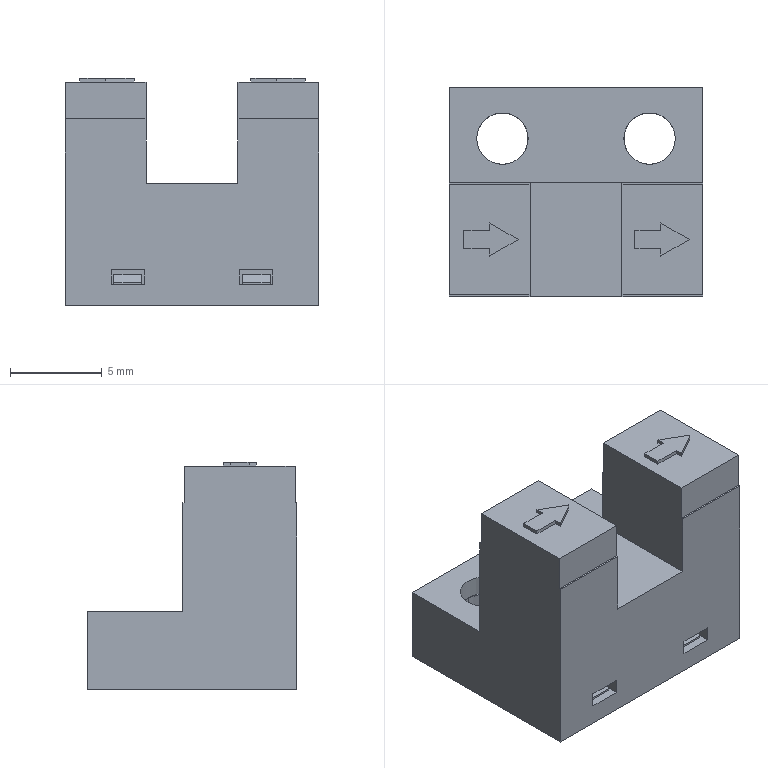Part | SolidWorks | features BaseBody 2 | 2 solids | 162 faces | box 13.8 x 11.4 x 12.35 mm | volume 654.662 mm3 | plane 148 | cylinder 11 | spline 3 | commonest cylinder face diameters 2.8 x8 3 x3